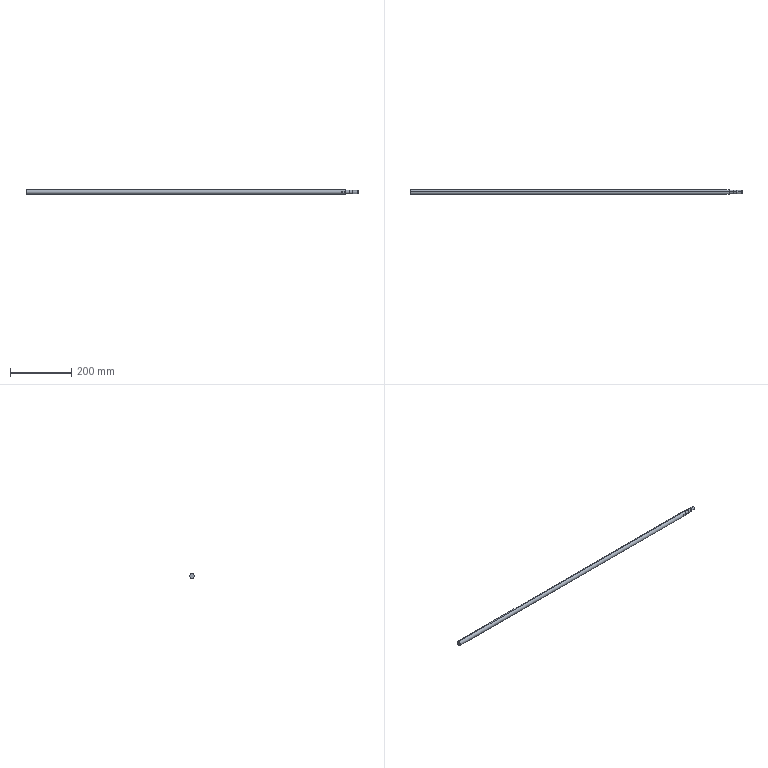Part | SolidWorks | features BaseBody 1 | 1 solid | 26 faces | box 1084 x 15 x 15 mm | volume 188228 mm3 | plane 12 | cylinder 10 | cone 4 | commonest cylinder face diameters 10 x2 10.5 x2 11.9 x2 12 x2 15 x2
STEP:
#1=CARTESIAN_POINT('',(1037.,7.,2.693));
#2=VERTEX_POINT('',#1);
#3=CARTESIAN_POINT('',(1037.,7.,-2.693));
#4=VERTEX_POINT('',#3);
#5=CARTESIAN_POINT('',(1037.,0.,0.));
#6=DIRECTION('',(-1.,0.,0.));
#7=DIRECTION('',(0.,0.,1.));
#8=AXIS2_PLACEMENT_3D('',#5,#6,#7);
#9=CIRCLE('',#8,7.5);
#10=EDGE_CURVE('',#2,#4,#9,.T.);
#11=ORIENTED_EDGE('',*,*,#10,.T.);
#12=CARTESIAN_POINT('',(1045.,7.,-2.693));
#13=VERTEX_POINT('',#12);
#14=CARTESIAN_POINT('',(-1000.,7.,-2.693));
#15=DIRECTION('',(1.,0.,0.));
#16=VECTOR('',#15,1000.);
#17=LINE('',#14,#16);
#18=EDGE_CURVE('',#4,#13,#17,.T.);
#19=ORIENTED_EDGE('',*,*,#18,.T.);
#20=CARTESIAN_POINT('',(1045.,7.,2.693));
#21=VERTEX_POINT('',#20);
#22=CARTESIAN_POINT('',(1045.,0.,0.));
#23=DIRECTION('',(1.,0.,0.));
#24=DIRECTION('',(0.,0.,1.));
#25=AXIS2_PLACEMENT_3D('',#22,#23,#24);
#26=CIRCLE('',#25,7.5);
#27=EDGE_CURVE('',#13,#21,#26,.T.);
#28=ORIENTED_EDGE('',*,*,#27,.T.);
#29=CARTESIAN_POINT('',(-1000.,7.,2.693));
#30=DIRECTION('',(-1.,0.,0.));
#31=VECTOR('',#30,1000.);
#32=LINE('',#29,#31);
#33=EDGE_CURVE('',#21,#2,#32,.T.);
#34=ORIENTED_EDGE('',*,*,#33,.T.);
#35=EDGE_LOOP('',(#11,#19,#28,#34));
#36=FACE_BOUND('',#35,.T.);
#37=CARTESIAN_POINT('',(1048.,0.,7.5));
#38=VERTEX_POINT('',#37);
#39=CARTESIAN_POINT('',(1048.,0.,-7.5));
#40=VERTEX_POINT('',#39);
#41=CARTESIAN_POINT('',(1048.,0.,0.));
#42=DIRECTION('',(-1.,0.,0.));
#43=DIRECTION('',(0.,0.,1.));
#44=AXIS2_PLACEMENT_3D('',#41,#42,#43);
#45=CIRCLE('',#44,7.5);
#46=EDGE_CURVE('',#38,#40,#45,.T.);
#47=ORIENTED_EDGE('',*,*,#46,.T.);
#48=CARTESIAN_POINT('',(6.,0.,-7.5));
#49=VERTEX_POINT('',#48);
#50=CARTESIAN_POINT('',(-1000.,0.,-7.5));
#51=DIRECTION('',(-1.,0.,0.));
#52=VECTOR('',#51,1000.);
#53=LINE('',#50,#52);
#54=EDGE_CURVE('',#40,#49,#53,.T.);
#55=ORIENTED_EDGE('',*,*,#54,.T.);
#56=CARTESIAN_POINT('',(6.,0.,7.5));
#57=VERTEX_POINT('',#56);
#58=CARTESIAN_POINT('',(6.,0.,0.));
#59=DIRECTION('',(1.,0.,0.));
#60=DIRECTION('',(0.,0.,1.));
#61=AXIS2_PLACEMENT_3D('',#58,#59,#60);
#62=CIRCLE('',#61,7.5);
#63=EDGE_CURVE('',#49,#57,#62,.T.);
#64=ORIENTED_EDGE('',*,*,#63,.T.);
#65=CARTESIAN_POINT('',(-1000.,0.,7.5));
#66=DIRECTION('',(-1.,0.,0.));
#67=VECTOR('',#66,1000.);
#68=LINE('',#65,#67);
#69=EDGE_CURVE('',#38,#57,#68,.T.);
#70=ORIENTED_EDGE('',*,*,#69,.F.);
#71=EDGE_LOOP('',(#47,#55,#64,#70));
#72=FACE_OUTER_BOUND('',#71,.T.);
#73=CARTESIAN_POINT('',(-1000.,0.,0.));
#74=DIRECTION('',(-1.,0.,0.));
#75=DIRECTION('',(0.,0.,1.));
#76=AXIS2_PLACEMENT_3D('',#73,#74,#75);
#77=CYLINDRICAL_SURFACE('',#76,7.5);
#78=ADVANCED_FACE('',(#36,#72),#77,.T.);
#79=CARTESIAN_POINT('',(1062.,0.,6.));
#80=VERTEX_POINT('',#79);
#81=CARTESIAN_POINT('',(1062.,0.,-6.));
#82=VERTEX_POINT('',#81);
#83=CARTESIAN_POINT('',(1062.,0.,0.));
#84=DIRECTION('',(-1.,0.,0.));
#85=DIRECTION('',(0.,0.,1.));
#86=AXIS2_PLACEMENT_3D('',#83,#84,#85);
#87=CIRCLE('',#86,6.);
#88=EDGE_CURVE('',#80,#82,#87,.T.);
#89=ORIENTED_EDGE('',*,*,#88,.T.);
#90=CARTESIAN_POINT('',(1048.,0.,-6.));
#91=VERTEX_POINT('',#90);
#92=CARTESIAN_POINT('',(-1000.,0.,-6.));
#93=DIRECTION('',(-1.,0.,0.));
#94=VECTOR('',#93,1000.);
#95=LINE('',#92,#94);
#96=EDGE_CURVE('',#82,#91,#95,.T.);
#97=ORIENTED_EDGE('',*,*,#96,.T.);
#98=CARTESIAN_POINT('',(1048.,0.,6.));
#99=VERTEX_POINT('',#98);
#100=CARTESIAN_POINT('',(1048.,0.,0.));
#101=DIRECTION('',(1.,0.,0.));
#102=DIRECTION('',(0.,0.,1.));
#103=AXIS2_PLACEMENT_3D('',#100,#101,#102);
#104=CIRCLE('',#103,6.);
#105=EDGE_CURVE('',#91,#99,#104,.T.);
#106=ORIENTED_EDGE('',*,*,#105,.T.);
#107=CARTESIAN_POINT('',(-1000.,0.,6.));
#108=DIRECTION('',(-1.,0.,0.));
#109=VECTOR('',#108,1000.);
#110=LINE('',#107,#109);
#111=EDGE_CURVE('',#80,#99,#110,.T.);
#112=ORIENTED_EDGE('',*,*,#111,.F.);
#113=EDGE_LOOP('',(#89,#97,#106,#112));
#114=FACE_OUTER_BOUND('',#113,.T.);
#115=CARTESIAN_POINT('',(-1000.,0.,0.));
#116=DIRECTION('',(-1.,0.,0.));
#117=DIRECTION('',(0.,0.,1.));
#118=AXIS2_PLACEMENT_3D('',#115,#116,#117);
#119=CYLINDRICAL_SURFACE('',#118,6.);
#120=ADVANCED_FACE('',(#114),#119,.T.);
#121=CARTESIAN_POINT('',(1062.,0.,5.95));
#122=VERTEX_POINT('',#121);
#123=CARTESIAN_POINT('',(1062.,0.,-5.95));
#124=VERTEX_POINT('',#123);
#125=CARTESIAN_POINT('',(1062.,0.,0.));
#126=DIRECTION('',(-1.,0.,0.));
#127=DIRECTION('',(0.,0.,-1.));
#128=AXIS2_PLACEMENT_3D('',#125,#126,#127);
#129=CIRCLE('',#128,5.95);
#130=EDGE_CURVE('',#122,#124,#129,.T.);
#131=ORIENTED_EDGE('',*,*,#130,.F.);
#132=CARTESIAN_POINT('',(1071.8,0.,5.95));
#133=VERTEX_POINT('',#132);
#134=CARTESIAN_POINT('',(1062.,0.,5.95));
#135=DIRECTION('',(1.,0.,0.));
#136=VECTOR('',#135,1000.);
#137=LINE('',#134,#136);
#138=EDGE_CURVE('',#122,#133,#137,.T.);
#139=ORIENTED_EDGE('',*,*,#138,.T.);
#140=CARTESIAN_POINT('',(1071.8,0.,-5.95));
#141=VERTEX_POINT('',#140);
#142=CARTESIAN_POINT('',(1071.8,0.,0.));
#143=DIRECTION('',(-1.,0.,0.));
#144=DIRECTION('',(0.,0.,-1.));
#145=AXIS2_PLACEMENT_3D('',#142,#143,#144);
#146=CIRCLE('',#145,5.95);
#147=EDGE_CURVE('',#133,#141,#146,.T.);
#148=ORIENTED_EDGE('',*,*,#147,.T.);
#149=CARTESIAN_POINT('',(1062.,0.,-5.95));
#150=DIRECTION('',(1.,0.,0.));
#151=VECTOR('',#150,1000.);
#152=LINE('',#149,#151);
#153=EDGE_CURVE('',#124,#141,#152,.T.);
#154=ORIENTED_EDGE('',*,*,#153,.F.);
#155=EDGE_LOOP('',(#131,#139,#148,#154));
#156=FACE_OUTER_BOUND('',#155,.T.);
#157=CARTESIAN_POINT('',(1062.,0.,0.));
#158=DIRECTION('',(1.,0.,0.));
#159=DIRECTION('',(0.,0.,-1.));
#160=AXIS2_PLACEMENT_3D('',#157,#158,#159);
#161=CYLINDRICAL_SURFACE('',#160,5.95);
#162=ADVANCED_FACE('',(#156),#161,.T.);
#163=CARTESIAN_POINT('',(1072.,0.,5.75));
#164=VERTEX_POINT('',#163);
#165=CARTESIAN_POINT('',(1072.,0.,-5.75));
#166=VERTEX_POINT('',#165);
#167=CARTESIAN_POINT('',(1072.,0.,0.));
#168=DIRECTION('',(-1.,0.,0.));
#169=DIRECTION('',(0.,0.,1.));
#170=AXIS2_PLACEMENT_3D('',#167,#168,#169);
#171=CIRCLE('',#170,5.75);
#172=EDGE_CURVE('',#164,#166,#171,.T.);
#173=ORIENTED_EDGE('',*,*,#172,.T.);
#174=CARTESIAN_POINT('',(1071.8,0.,-5.95));
#175=DIRECTION('',(-0.7071,0.,-0.7071));
#176=VECTOR('',#175,1000.);
#177=LINE('',#174,#176);
#178=EDGE_CURVE('',#166,#141,#177,.T.);
#179=ORIENTED_EDGE('',*,*,#178,.T.);
#180=ORIENTED_EDGE('',*,*,#147,.F.);
#181=CARTESIAN_POINT('',(1071.8,0.,5.95));
#182=DIRECTION('',(-0.7071,0.,0.7071));
#183=VECTOR('',#182,1000.);
#184=LINE('',#181,#183);
#185=EDGE_CURVE('',#164,#133,#184,.T.);
#186=ORIENTED_EDGE('',*,*,#185,.F.);
#187=EDGE_LOOP('',(#173,#179,#180,#186));
#188=FACE_OUTER_BOUND('',#187,.T.);
#189=CARTESIAN_POINT('',(1071.8,0.,0.));
#190=DIRECTION('',(-1.,0.,0.));
#191=DIRECTION('',(0.,0.,1.));
#192=AXIS2_PLACEMENT_3D('',#189,#190,#191);
#193=CONICAL_SURFACE('',#192,5.95,0.7854);
#194=ADVANCED_FACE('',(#188),#193,.T.);
#195=CARTESIAN_POINT('',(1073.5,0.,5.25));
#196=VERTEX_POINT('',#195);
#197=CARTESIAN_POINT('',(1073.5,0.,-5.25));
#198=VERTEX_POINT('',#197);
#199=CARTESIAN_POINT('',(1073.5,0.,0.));
#200=DIRECTION('',(-1.,0.,0.));
#201=DIRECTION('',(0.,0.,1.));
#202=AXIS2_PLACEMENT_3D('',#199,#200,#201);
#203=CIRCLE('',#202,5.25);
#204=EDGE_CURVE('',#196,#198,#203,.T.);
#205=ORIENTED_EDGE('',*,*,#204,.T.);
#206=CARTESIAN_POINT('',(1072.,0.,-5.25));
#207=VERTEX_POINT('',#206);
#208=CARTESIAN_POINT('',(-1000.,0.,-5.25));
#209=DIRECTION('',(-1.,0.,0.));
#210=VECTOR('',#209,1000.);
#211=LINE('',#208,#210);
#212=EDGE_CURVE('',#198,#207,#211,.T.);
#213=ORIENTED_EDGE('',*,*,#212,.T.);
#214=CARTESIAN_POINT('',(1072.,0.,5.25));
#215=VERTEX_POINT('',#214);
#216=CARTESIAN_POINT('',(1072.,0.,0.));
#217=DIRECTION('',(1.,0.,0.));
#218=DIRECTION('',(0.,0.,1.));
#219=AXIS2_PLACEMENT_3D('',#216,#217,#218);
#220=CIRCLE('',#219,5.25);
#221=EDGE_CURVE('',#207,#215,#220,.T.);
#222=ORIENTED_EDGE('',*,*,#221,.T.);
#223=CARTESIAN_POINT('',(-1000.,0.,5.25));
#224=DIRECTION('',(-1.,0.,0.));
#225=VECTOR('',#224,1000.);
#226=LINE('',#223,#225);
#227=EDGE_CURVE('',#196,#215,#226,.T.);
#228=ORIENTED_EDGE('',*,*,#227,.F.);
#229=EDGE_LOOP('',(#205,#213,#222,#228));
#230=FACE_OUTER_BOUND('',#229,.T.);
#231=CARTESIAN_POINT('',(-1000.,0.,0.));
#232=DIRECTION('',(-1.,0.,0.));
#233=DIRECTION('',(0.,0.,1.));
#234=AXIS2_PLACEMENT_3D('',#231,#232,#233);
#235=CYLINDRICAL_SURFACE('',#234,5.25);
#236=ADVANCED_FACE('',(#230),#235,.T.);
#237=CARTESIAN_POINT('',(1089.8,0.,5.));
#238=VERTEX_POINT('',#237);
#239=CARTESIAN_POINT('',(1089.8,0.,-5.));
#240=VERTEX_POINT('',#239);
#241=CARTESIAN_POINT('',(1089.8,0.,0.));
#242=DIRECTION('',(-1.,0.,0.));
#243=DIRECTION('',(0.,0.,1.));
#244=AXIS2_PLACEMENT_3D('',#241,#242,#243);
#245=CIRCLE('',#244,5.);
#246=EDGE_CURVE('',#238,#240,#245,.T.);
#247=ORIENTED_EDGE('',*,*,#246,.T.);
#248=CARTESIAN_POINT('',(1073.5,0.,-5.));
#249=VERTEX_POINT('',#248);
#250=CARTESIAN_POINT('',(-1000.,0.,-5.));
#251=DIRECTION('',(-1.,0.,0.));
#252=VECTOR('',#251,1000.);
#253=LINE('',#250,#252);
#254=EDGE_CURVE('',#240,#249,#253,.T.);
#255=ORIENTED_EDGE('',*,*,#254,.T.);
#256=CARTESIAN_POINT('',(1073.5,0.,5.));
#257=VERTEX_POINT('',#256);
#258=CARTESIAN_POINT('',(1073.5,0.,0.));
#259=DIRECTION('',(1.,0.,0.));
#260=DIRECTION('',(0.,0.,1.));
#261=AXIS2_PLACEMENT_3D('',#258,#259,#260);
#262=CIRCLE('',#261,5.);
#263=EDGE_CURVE('',#249,#257,#262,.T.);
#264=ORIENTED_EDGE('',*,*,#263,.T.);
#265=CARTESIAN_POINT('',(-1000.,0.,5.));
#266=DIRECTION('',(-1.,0.,0.));
#267=VECTOR('',#266,1000.);
#268=LINE('',#265,#267);
#269=EDGE_CURVE('',#238,#257,#268,.T.);
#270=ORIENTED_EDGE('',*,*,#269,.F.);
#271=EDGE_LOOP('',(#247,#255,#264,#270));
#272=FACE_OUTER_BOUND('',#271,.T.);
#273=CARTESIAN_POINT('',(-1000.,0.,0.));
#274=DIRECTION('',(-1.,0.,0.));
#275=DIRECTION('',(0.,0.,1.));
#276=AXIS2_PLACEMENT_3D('',#273,#274,#275);
#277=CYLINDRICAL_SURFACE('',#276,5.);
#278=ADVANCED_FACE('',(#272),#277,.T.);
#279=CARTESIAN_POINT('',(1090.,0.,4.8));
#280=VERTEX_POINT('',#279);
#281=CARTESIAN_POINT('',(1090.,0.,-4.8));
#282=VERTEX_POINT('',#281);
#283=CARTESIAN_POINT('',(1090.,0.,0.));
#284=DIRECTION('',(-1.,0.,0.));
#285=DIRECTION('',(0.,0.,1.));
#286=AXIS2_PLACEMENT_3D('',#283,#284,#285);
#287=CIRCLE('',#286,4.8);
#288=EDGE_CURVE('',#280,#282,#287,.T.);
#289=ORIENTED_EDGE('',*,*,#288,.T.);
#290=CARTESIAN_POINT('',(1089.8,0.,-5.));
#291=DIRECTION('',(-0.7071,0.,-0.7071));
#292=VECTOR('',#291,1000.);
#293=LINE('',#290,#292);
#294=EDGE_CURVE('',#282,#240,#293,.T.);
#295=ORIENTED_EDGE('',*,*,#294,.T.);
#296=ORIENTED_EDGE('',*,*,#246,.F.);
#297=CARTESIAN_POINT('',(1089.8,0.,5.));
#298=DIRECTION('',(-0.7071,0.,0.7071));
#299=VECTOR('',#298,1000.);
#300=LINE('',#297,#299);
#301=EDGE_CURVE('',#280,#238,#300,.T.);
#302=ORIENTED_EDGE('',*,*,#301,.F.);
#303=EDGE_LOOP('',(#289,#295,#296,#302));
#304=FACE_OUTER_BOUND('',#303,.T.);
#305=CARTESIAN_POINT('',(1089.8,0.,0.));
#306=DIRECTION('',(-1.,0.,0.));
#307=DIRECTION('',(0.,0.,1.));
#308=AXIS2_PLACEMENT_3D('',#305,#306,#307);
#309=CONICAL_SURFACE('',#308,5.,0.7854);
#310=ADVANCED_FACE('',(#304),#309,.T.);
#311=ORIENTED_EDGE('',*,*,#54,.F.);
#312=CARTESIAN_POINT('',(1048.,0.,0.));
#313=DIRECTION('',(-1.,0.,0.));
#314=DIRECTION('',(0.,0.,1.));
#315=AXIS2_PLACEMENT_3D('',#312,#313,#314);
#316=CIRCLE('',#315,7.5);
#317=EDGE_CURVE('',#40,#38,#316,.T.);
#318=ORIENTED_EDGE('',*,*,#317,.T.);
#319=ORIENTED_EDGE('',*,*,#69,.T.);
#320=CARTESIAN_POINT('',(6.,0.,0.));
#321=DIRECTION('',(1.,0.,0.));
#322=DIRECTION('',(0.,0.,1.));
#323=AXIS2_PLACEMENT_3D('',#320,#321,#322);
#324=CIRCLE('',#323,7.5);
#325=EDGE_CURVE('',#57,#49,#324,.T.);
#326=ORIENTED_EDGE('',*,*,#325,.T.);
#327=EDGE_LOOP('',(#311,#318,#319,#326));
#328=FACE_OUTER_BOUND('',#327,.T.);
#329=CARTESIAN_POINT('',(1045.,-7.,-2.693));
#330=VERTEX_POINT('',#329);
#331=CARTESIAN_POINT('',(1037.,-7.,-2.693));
#332=VERTEX_POINT('',#331);
#333=CARTESIAN_POINT('',(-1000.,-7.,-2.693));
#334=DIRECTION('',(-1.,0.,0.));
#335=VECTOR('',#334,1000.);
#336=LINE('',#333,#335);
#337=EDGE_CURVE('',#330,#332,#336,.T.);
#338=ORIENTED_EDGE('',*,*,#337,.T.);
#339=CARTESIAN_POINT('',(1037.,-7.,2.693));
#340=VERTEX_POINT('',#339);
#341=CARTESIAN_POINT('',(1037.,0.,0.));
#342=DIRECTION('',(-1.,0.,0.));
#343=DIRECTION('',(0.,0.,1.));
#344=AXIS2_PLACEMENT_3D('',#341,#342,#343);
#345=CIRCLE('',#344,7.5);
#346=EDGE_CURVE('',#332,#340,#345,.T.);
#347=ORIENTED_EDGE('',*,*,#346,.T.);
#348=CARTESIAN_POINT('',(1045.,-7.,2.693));
#349=VERTEX_POINT('',#348);
#350=CARTESIAN_POINT('',(-1000.,-7.,2.693));
#351=DIRECTION('',(1.,0.,0.));
#352=VECTOR('',#351,1000.);
#353=LINE('',#350,#352);
#354=EDGE_CURVE('',#340,#349,#353,.T.);
#355=ORIENTED_EDGE('',*,*,#354,.T.);
#356=CARTESIAN_POINT('',(1045.,0.,0.));
#357=DIRECTION('',(1.,0.,0.));
#358=DIRECTION('',(0.,0.,1.));
#359=AXIS2_PLACEMENT_3D('',#356,#357,#358);
#360=CIRCLE('',#359,7.5);
#361=EDGE_CURVE('',#349,#330,#360,.T.);
#362=ORIENTED_EDGE('',*,*,#361,.T.);
#363=EDGE_LOOP('',(#338,#347,#355,#362));
#364=FACE_BOUND('',#363,.T.);
#365=CARTESIAN_POINT('',(-1000.,0.,0.));
#366=DIRECTION('',(-1.,0.,0.));
#367=DIRECTION('',(0.,0.,1.));
#368=AXIS2_PLACEMENT_3D('',#365,#366,#367);
#369=CYLINDRICAL_SURFACE('',#368,7.5);
#370=ADVANCED_FACE('',(#328,#364),#369,.T.);
#371=ORIENTED_EDGE('',*,*,#325,.F.);
#372=ORIENTED_EDGE('',*,*,#63,.F.);
#373=EDGE_LOOP('',(#371,#372));
#374=FACE_OUTER_BOUND('',#373,.T.);
#375=CARTESIAN_POINT('',(6.,5.,0.));
#376=DIRECTION('',(1.,0.,0.));
#377=DIRECTION('',(0.,0.,-1.));
#378=AXIS2_PLACEMENT_3D('',#375,#376,#377);
#379=PLANE('',#378);
#380=ADVANCED_FACE('',(#374),#379,.F.);
#381=CARTESIAN_POINT('',(1048.,0.,0.));
#382=DIRECTION('',(1.,0.,0.));
#383=DIRECTION('',(0.,0.,1.));
#384=AXIS2_PLACEMENT_3D('',#381,#382,#383);
#385=CIRCLE('',#384,6.);
#386=EDGE_CURVE('',#99,#91,#385,.T.);
#387=ORIENTED_EDGE('',*,*,#386,.F.);
#388=ORIENTED_EDGE('',*,*,#105,.F.);
#389=EDGE_LOOP('',(#387,#388));
#390=FACE_BOUND('',#389,.T.);
#391=ORIENTED_EDGE('',*,*,#46,.F.);
#392=ORIENTED_EDGE('',*,*,#317,.F.);
#393=EDGE_LOOP('',(#391,#392));
#394=FACE_OUTER_BOUND('',#393,.T.);
#395=CARTESIAN_POINT('',(1048.,6.,0.));
#396=DIRECTION('',(-1.,0.,0.));
#397=DIRECTION('',(0.,0.,1.));
#398=AXIS2_PLACEMENT_3D('',#395,#396,#397);
#399=PLANE('',#398);
#400=ADVANCED_FACE('',(#390,#394),#399,.F.);
#401=ORIENTED_EDGE('',*,*,#18,.F.);
#402=CARTESIAN_POINT('',(1037.,7.,-5.));
#403=DIRECTION('',(0.,0.,-1.));
#404=VECTOR('',#403,1000.);
#405=LINE('',#402,#404);
#406=EDGE_CURVE('',#2,#4,#405,.T.);
#407=ORIENTED_EDGE('',*,*,#406,.F.);
#408=ORIENTED_EDGE('',*,*,#33,.F.);
#409=CARTESIAN_POINT('',(1045.,7.,-5.));
#410=DIRECTION('',(0.,0.,1.));
#411=VECTOR('',#410,1000.);
#412=LINE('',#409,#411);
#413=EDGE_CURVE('',#13,#21,#412,.T.);
#414=ORIENTED_EDGE('',*,*,#413,.F.);
#415=EDGE_LOOP('',(#401,#407,#408,#414));
#416=FACE_OUTER_BOUND('',#415,.T.);
#417=CARTESIAN_POINT('',(1037.,7.,-5.));
#418=DIRECTION('',(0.,-1.,0.));
#419=DIRECTION('',(0.,0.,-1.));
#420=AXIS2_PLACEMENT_3D('',#417,#418,#419);
#421=PLANE('',#420);
#422=ADVANCED_FACE('',(#416),#421,.F.);
#423=ORIENTED_EDGE('',*,*,#10,.F.);
#424=ORIENTED_EDGE('',*,*,#406,.T.);
#425=EDGE_LOOP('',(#423,#424));
#426=FACE_OUTER_BOUND('',#425,.T.);
#427=CARTESIAN_POINT('',(1037.,7.5,-5.));
#428=DIRECTION('',(-1.,0.,0.));
#429=DIRECTION('',(0.,0.,1.));
#430=AXIS2_PLACEMENT_3D('',#427,#428,#429);
#431=PLANE('',#430);
#432=ADVANCED_FACE('',(#426),#431,.F.);
#433=ORIENTED_EDGE('',*,*,#27,.F.);
#434=ORIENTED_EDGE('',*,*,#413,.T.);
#435=EDGE_LOOP('',(#433,#434));
#436=FACE_OUTER_BOUND('',#435,.T.);
#437=CARTESIAN_POINT('',(1045.,7.5,-5.));
#438=DIRECTION('',(1.,0.,0.));
#439=DIRECTION('',(0.,0.,-1.));
#440=AXIS2_PLACEMENT_3D('',#437,#438,#439);
#441=PLANE('',#440);
#442=ADVANCED_FACE('',(#436),#441,.F.);
#443=ORIENTED_EDGE('',*,*,#346,.F.);
#444=CARTESIAN_POINT('',(1037.,-7.,-5.));
#445=DIRECTION('',(0.,0.,-1.));
#446=VECTOR('',#445,1000.);
#447=LINE('',#444,#446);
#448=EDGE_CURVE('',#340,#332,#447,.T.);
#449=ORIENTED_EDGE('',*,*,#448,.F.);
#450=EDGE_LOOP('',(#443,#449));
#451=FACE_OUTER_BOUND('',#450,.T.);
#452=CARTESIAN_POINT('',(1037.,-7.5,-5.));
#453=DIRECTION('',(-1.,0.,0.));
#454=DIRECTION('',(0.,0.,1.));
#455=AXIS2_PLACEMENT_3D('',#452,#453,#454);
#456=PLANE('',#455);
#457=ADVANCED_FACE('',(#451),#456,.F.);
#458=ORIENTED_EDGE('',*,*,#354,.F.);
#459=ORIENTED_EDGE('',*,*,#448,.T.);
#460=ORIENTED_EDGE('',*,*,#337,.F.);
#461=CARTESIAN_POINT('',(1045.,-7.,-5.));
#462=DIRECTION('',(0.,0.,-1.));
#463=VECTOR('',#462,1000.);
#464=LINE('',#461,#463);
#465=EDGE_CURVE('',#349,#330,#464,.T.);
#466=ORIENTED_EDGE('',*,*,#465,.F.);
#467=EDGE_LOOP('',(#458,#459,#460,#466));
#468=FACE_OUTER_BOUND('',#467,.T.);
#469=CARTESIAN_POINT('',(1037.,-7.,-5.));
#470=DIRECTION('',(0.,1.,0.));
#471=DIRECTION('',(0.,0.,1.));
#472=AXIS2_PLACEMENT_3D('',#469,#470,#471);
#473=PLANE('',#472);
#474=ADVANCED_FACE('',(#468),#473,.F.);
#475=ORIENTED_EDGE('',*,*,#361,.F.);
#476=ORIENTED_EDGE('',*,*,#465,.T.);
#477=EDGE_LOOP('',(#475,#476));
#478=FACE_OUTER_BOUND('',#477,.T.);
#479=CARTESIAN_POINT('',(1045.,-7.5,-5.));
#480=DIRECTION('',(1.,0.,0.));
#481=DIRECTION('',(0.,0.,-1.));
#482=AXIS2_PLACEMENT_3D('',#479,#480,#481);
#483=PLANE('',#482);
#484=ADVANCED_FACE('',(#478),#483,.F.);
#485=ORIENTED_EDGE('',*,*,#96,.F.);
#486=CARTESIAN_POINT('',(1062.,0.,0.));
#487=DIRECTION('',(-1.,0.,0.));
#488=DIRECTION('',(0.,0.,1.));
#489=AXIS2_PLACEMENT_3D('',#486,#487,#488);
#490=CIRCLE('',#489,6.);
#491=EDGE_CURVE('',#82,#80,#490,.T.);
#492=ORIENTED_EDGE('',*,*,#491,.T.);
#493=ORIENTED_EDGE('',*,*,#111,.T.);
#494=ORIENTED_EDGE('',*,*,#386,.T.);
#495=EDGE_LOOP('',(#485,#492,#493,#494));
#496=FACE_OUTER_BOUND('',#495,.T.);
#497=CARTESIAN_POINT('',(-1000.,0.,0.));
#498=DIRECTION('',(-1.,0.,0.));
#499=DIRECTION('',(0.,0.,1.));
#500=AXIS2_PLACEMENT_3D('',#497,#498,#499);
#501=CYLINDRICAL_SURFACE('',#500,6.);
#502=ADVANCED_FACE('',(#496),#501,.T.);
#503=ORIENTED_EDGE('',*,*,#88,.F.);
#504=ORIENTED_EDGE('',*,*,#491,.F.);
#505=EDGE_LOOP('',(#503,#504));
#506=FACE_OUTER_BOUND('',#505,.T.);
#507=CARTESIAN_POINT('',(1062.,0.,0.));
#508=DIRECTION('',(-1.,0.,0.));
#509=DIRECTION('',(0.,0.,-1.));
#510=AXIS2_PLACEMENT_3D('',#507,#508,#509);
#511=CIRCLE('',#510,5.95);
#512=EDGE_CURVE('',#124,#122,#511,.T.);
#513=ORIENTED_EDGE('',*,*,#512,.T.);
#514=ORIENTED_EDGE('',*,*,#130,.T.);
#515=EDGE_LOOP('',(#513,#514));
#516=FACE_BOUND('',#515,.T.);
#517=CARTESIAN_POINT('',(1062.,0.,0.));
#518=DIRECTION('',(1.,0.,0.));
#519=DIRECTION('',(0.,0.,-1.));
#520=AXIS2_PLACEMENT_3D('',#517,#518,#519);
#521=PLANE('',#520);
#522=ADVANCED_FACE('',(#506,#516),#521,.T.);
#523=ORIENTED_EDGE('',*,*,#138,.F.);
#524=ORIENTED_EDGE('',*,*,#512,.F.);
#525=ORIENTED_EDGE('',*,*,#153,.T.);
#526=CARTESIAN_POINT('',(1071.8,0.,0.));
#527=DIRECTION('',(-1.,0.,0.));
#528=DIRECTION('',(0.,0.,-1.));
#529=AXIS2_PLACEMENT_3D('',#526,#527,#528);
#530=CIRCLE('',#529,5.95);
#531=EDGE_CURVE('',#141,#133,#530,.T.);
#532=ORIENTED_EDGE('',*,*,#531,.T.);
#533=EDGE_LOOP('',(#523,#524,#525,#532));
#534=FACE_OUTER_BOUND('',#533,.T.);
#535=CARTESIAN_POINT('',(1062.,0.,0.));
#536=DIRECTION('',(1.,0.,0.));
#537=DIRECTION('',(0.,0.,-1.));
#538=AXIS2_PLACEMENT_3D('',#535,#536,#537);
#539=CYLINDRICAL_SURFACE('',#538,5.95);
#540=ADVANCED_FACE('',(#534),#539,.T.);
#541=ORIENTED_EDGE('',*,*,#178,.F.);
#542=CARTESIAN_POINT('',(1072.,0.,0.));
#543=DIRECTION('',(-1.,0.,0.));
#544=DIRECTION('',(0.,0.,1.));
#545=AXIS2_PLACEMENT_3D('',#542,#543,#544);
#546=CIRCLE('',#545,5.75);
#547=EDGE_CURVE('',#166,#164,#546,.T.);
#548=ORIENTED_EDGE('',*,*,#547,.T.);
#549=ORIENTED_EDGE('',*,*,#185,.T.);
#550=ORIENTED_EDGE('',*,*,#531,.F.);
#551=EDGE_LOOP('',(#541,#548,#549,#550));
#552=FACE_OUTER_BOUND('',#551,.T.);
#553=CARTESIAN_POINT('',(1071.8,0.,0.));
#554=DIRECTION('',(-1.,0.,0.));
#555=DIRECTION('',(0.,0.,1.));
#556=AXIS2_PLACEMENT_3D('',#553,#554,#555);
#557=CONICAL_SURFACE('',#556,5.95,0.7854);
#558=ADVANCED_FACE('',(#552),#557,.T.);
#559=CARTESIAN_POINT('',(1072.,0.,0.));
#560=DIRECTION('',(1.,0.,0.));
#561=DIRECTION('',(0.,0.,1.));
#562=AXIS2_PLACEMENT_3D('',#559,#560,#561);
#563=CIRCLE('',#562,5.25);
#564=EDGE_CURVE('',#215,#207,#563,.T.);
#565=ORIENTED_EDGE('',*,*,#564,.F.);
#566=ORIENTED_EDGE('',*,*,#221,.F.);
#567=EDGE_LOOP('',(#565,#566));
#568=FACE_BOUND('',#567,.T.);
#569=ORIENTED_EDGE('',*,*,#172,.F.);
#570=ORIENTED_EDGE('',*,*,#547,.F.);
#571=EDGE_LOOP('',(#569,#570));
#572=FACE_OUTER_BOUND('',#571,.T.);
#573=CARTESIAN_POINT('',(1072.,6.,0.));
#574=DIRECTION('',(-1.,0.,0.));
#575=DIRECTION('',(0.,0.,1.));
#576=AXIS2_PLACEMENT_3D('',#573,#574,#575);
#577=PLANE('',#576);
#578=ADVANCED_FACE('',(#568,#572),#577,.F.);
#579=ORIENTED_EDGE('',*,*,#212,.F.);
#580=CARTESIAN_POINT('',(1073.5,0.,0.));
#581=DIRECTION('',(-1.,0.,0.));
#582=DIRECTION('',(0.,0.,1.));
#583=AXIS2_PLACEMENT_3D('',#580,#581,#582);
#584=CIRCLE('',#583,5.25);
#585=EDGE_CURVE('',#198,#196,#584,.T.);
#586=ORIENTED_EDGE('',*,*,#585,.T.);
#587=ORIENTED_EDGE('',*,*,#227,.T.);
#588=ORIENTED_EDGE('',*,*,#564,.T.);
#589=EDGE_LOOP('',(#579,#586,#587,#588));
#590=FACE_OUTER_BOUND('',#589,.T.);
#591=CARTESIAN_POINT('',(-1000.,0.,0.));
#592=DIRECTION('',(-1.,0.,0.));
#593=DIRECTION('',(0.,0.,1.));
#594=AXIS2_PLACEMENT_3D('',#591,#592,#593);
#595=CYLINDRICAL_SURFACE('',#594,5.25);
#596=ADVANCED_FACE('',(#590),#595,.T.);
#597=CARTESIAN_POINT('',(1073.5,0.,0.));
#598=DIRECTION('',(1.,0.,0.));
#599=DIRECTION('',(0.,0.,1.));
#600=AXIS2_PLACEMENT_3D('',#597,#598,#599);
#601=CIRCLE('',#600,5.);
#602=EDGE_CURVE('',#257,#249,#601,.T.);
#603=ORIENTED_EDGE('',*,*,#602,.F.);
#604=ORIENTED_EDGE('',*,*,#263,.F.);
#605=EDGE_LOOP('',(#603,#604));
#606=FACE_BOUND('',#605,.T.);
#607=ORIENTED_EDGE('',*,*,#204,.F.);
#608=ORIENTED_EDGE('',*,*,#585,.F.);
#609=EDGE_LOOP('',(#607,#608));
#610=FACE_OUTER_BOUND('',#609,.T.);
#611=CARTESIAN_POINT('',(1073.5,5.,0.));
#612=DIRECTION('',(-1.,0.,0.));
#613=DIRECTION('',(0.,0.,1.));
#614=AXIS2_PLACEMENT_3D('',#611,#612,#613);
#615=PLANE('',#614);
#616=ADVANCED_FACE('',(#606,#610),#615,.F.);
#617=ORIENTED_EDGE('',*,*,#254,.F.);
#618=CARTESIAN_POINT('',(1089.8,0.,0.));
#619=DIRECTION('',(-1.,0.,0.));
#620=DIRECTION('',(0.,0.,1.));
#621=AXIS2_PLACEMENT_3D('',#618,#619,#620);
#622=CIRCLE('',#621,5.);
#623=EDGE_CURVE('',#240,#238,#622,.T.);
#624=ORIENTED_EDGE('',*,*,#623,.T.);
#625=ORIENTED_EDGE('',*,*,#269,.T.);
#626=ORIENTED_EDGE('',*,*,#602,.T.);
#627=EDGE_LOOP('',(#617,#624,#625,#626));
#628=FACE_OUTER_BOUND('',#627,.T.);
#629=CARTESIAN_POINT('',(-1000.,0.,0.));
#630=DIRECTION('',(-1.,0.,0.));
#631=DIRECTION('',(0.,0.,1.));
#632=AXIS2_PLACEMENT_3D('',#629,#630,#631);
#633=CYLINDRICAL_SURFACE('',#632,5.);
#634=ADVANCED_FACE('',(#628),#633,.T.);
#635=ORIENTED_EDGE('',*,*,#294,.F.);
#636=CARTESIAN_POINT('',(1090.,0.,0.));
#637=DIRECTION('',(-1.,0.,0.));
#638=DIRECTION('',(0.,0.,1.));
#639=AXIS2_PLACEMENT_3D('',#636,#637,#638);
#640=CIRCLE('',#639,4.8);
#641=EDGE_CURVE('',#282,#280,#640,.T.);
#642=ORIENTED_EDGE('',*,*,#641,.T.);
#643=ORIENTED_EDGE('',*,*,#301,.T.);
#644=ORIENTED_EDGE('',*,*,#623,.F.);
#645=EDGE_LOOP('',(#635,#642,#643,#644));
#646=FACE_OUTER_BOUND('',#645,.T.);
#647=CARTESIAN_POINT('',(1089.8,0.,0.));
#648=DIRECTION('',(-1.,0.,0.));
#649=DIRECTION('',(0.,0.,1.));
#650=AXIS2_PLACEMENT_3D('',#647,#648,#649);
#651=CONICAL_SURFACE('',#650,5.,0.7854);
#652=ADVANCED_FACE('',(#646),#651,.T.);
#653=ORIENTED_EDGE('',*,*,#288,.F.);
#654=ORIENTED_EDGE('',*,*,#641,.F.);
#655=EDGE_LOOP('',(#653,#654));
#656=FACE_OUTER_BOUND('',#655,.T.);
#657=CARTESIAN_POINT('',(1090.,5.,0.));
#658=DIRECTION('',(-1.,0.,0.));
#659=DIRECTION('',(0.,0.,1.));
#660=AXIS2_PLACEMENT_3D('',#657,#658,#659);
#661=PLANE('',#660);
#662=ADVANCED_FACE('',(#656),#661,.F.);
#663=CLOSED_SHELL('',(#78,#120,#162,#194,#236,#278,#310,#370,#380,#400,#422,#432,#442,#457,#474,#484,#502,#522,#540,#558,#578,#596,#616,#634,#652,#662));
#664=MANIFOLD_SOLID_BREP('',#663);
#665=CARTESIAN_POINT('',(0.,0.,0.));
#666=DIRECTION('',(0.,0.,1.));
#667=DIRECTION('',(1.,0.,0.));
#668=AXIS2_PLACEMENT_3D('',#665,#666,#667);
#669=(LENGTH_UNIT()NAMED_UNIT(*)SI_UNIT(.MILLI.,.METRE.));
#670=UNCERTAINTY_MEASURE_WITH_UNIT(LENGTH_MEASURE(0.00001),#669,'','');
#671=(NAMED_UNIT(*)PLANE_ANGLE_UNIT()SI_UNIT($,.RADIAN.));
#672=(NAMED_UNIT(*)SI_UNIT($,.STERADIAN.)SOLID_ANGLE_UNIT());
#673=(GEOMETRIC_REPRESENTATION_CONTEXT(3)GLOBAL_UNCERTAINTY_ASSIGNED_CONTEXT((#670))GLOBAL_UNIT_ASSIGNED_CONTEXT((#669,#671,#672))REPRESENTATION_CONTEXT('',''));
#674=ADVANCED_BREP_SHAPE_REPRESENTATION('',(#664,#668),#673);